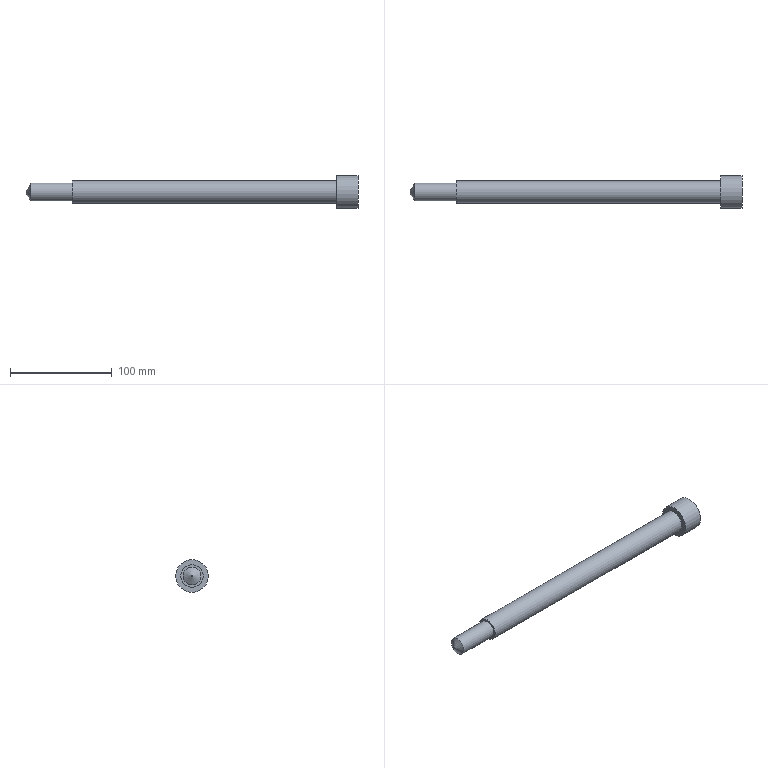Part | STEP file | solid 258 | 1 solid | 8 faces | box 325.5 x 32 x 32 mm | volume 125610 mm3 | plane 4 | cylinder 3 | cone 1 | commonest cylinder face diameters 17.5 x1 22 x1 32 x1